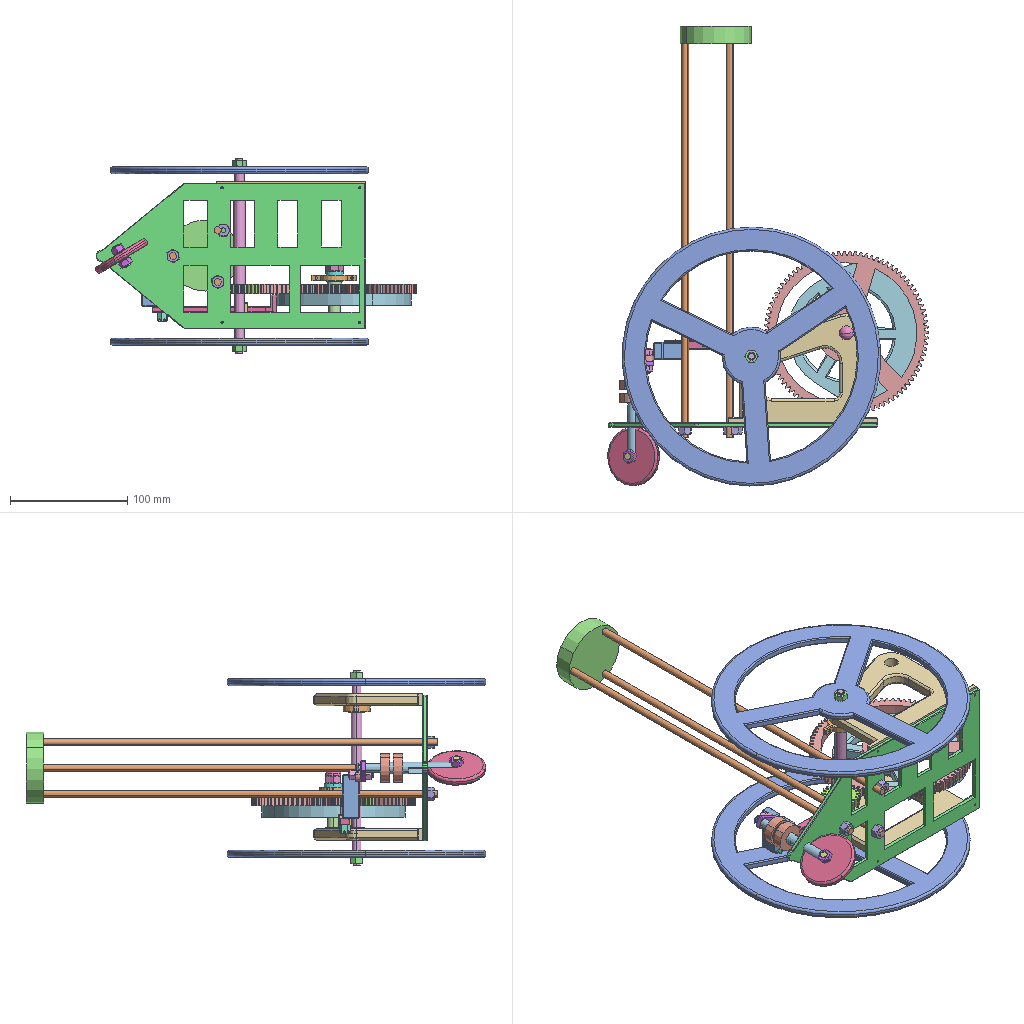Assembly | SolidWorks | 33 different items | 41 placed | box 273 x 391 x 166 mm
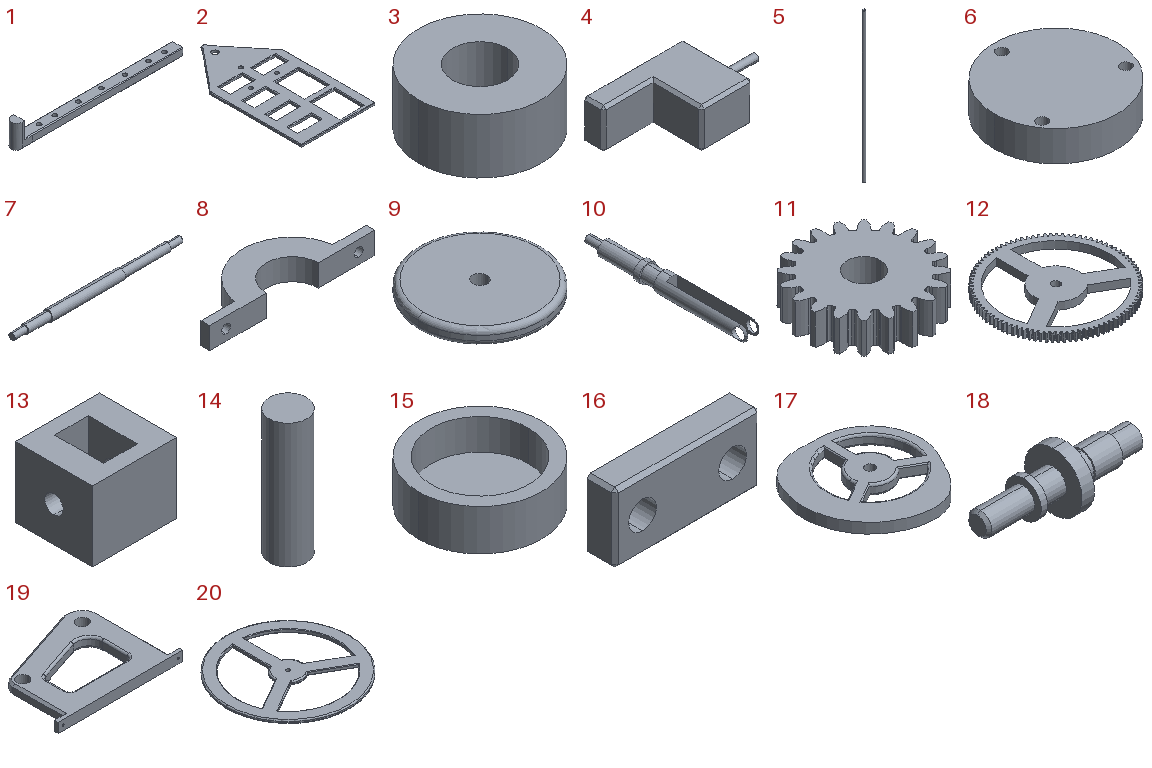Parts list (item | name | quantity | size | volume | features):
1 | - | x1 | 105.759 x 6.991 x 14.8 mm | 3589 mm3 | features Chamfer 1, Extrusion 1, Fillet 1, ICE 1
2 | - | x1 | 124.097 x 229.379 x 4 mm | 63027 mm3 | features Chamfer 8, Fillet 2, Extrusion 1, ICE 1
3 | - | x1 | 11.179 x 11.179 x 5 mm | 392.607 mm3 | features Extrusion 1
4 | - | x1 | 48 x 26.348 x 15 mm | 9753 mm3 | features Chamfer 1, Extrusion 1, ICE 1
5 | - | x3 | 6 x 6 x 350 mm | 9896 mm3 | features Extrusion 1
6 | - | x1 | 60.454 x 60.454 x 15 mm | 42106 mm3 | features Extrusion 1
7 | - | x1 | 166.354 x 10 x 10 mm | 9800 mm3 | features Revolution 1
8 | - | x4 | 38 x 11.5 x 5 mm | 894.544 mm3 | features ICE 2, Extrusion 1
9 | - | x1 | 50 x 50 x 6 mm | 11346 mm3 | features Extrusion 1, Fillet 1
10 | - | x1 | 10 x 90.414 x 10 mm | 3064 mm3 | features ICE 2, Revolution 1
11 | - | x1 | 32.74 x 32.74 x 8.27 mm | 5212 mm3 | features Extrusion 1
12 | - | x1 | 139.495 x 139.48 x 8.27 mm | 56874 mm3 | features Extrusion 1, ICE 1
13 | - | x1 | 11.98 x 10.98 x 10 mm | 942.243 mm3 | features Extrusion 1, ICE 1
14 | - | x1 | 6 x 6 x 20 mm | 565.487 mm3 | features Extrusion 1
15 | - | x2 | 24 x 24 x 8 mm | 1918 mm3 | features Extrusion 1, ICE 1
16 | - | x1 | 21 x 4 x 10 mm | 730.052 mm3 | features Chamfer 1, Extrusion 1, ICE 1
17 | - | x1 | 115.52 x 116.155 x 10 mm | 73313 mm3 | features Fillet 2, Chamfer 1, Extrusion 1, ICE 1
18 | - | x1 | 53.633 x 20 x 20 mm | 4453 mm3 | features Revolution 1
19 | - | x2 | 127.21 x 92.5 x 10 mm | 59705 mm3 | features Fillet 3, Chamfer 2, ICE 2, Extrusion 1
20 | - | x2 | 220.16 x 220.16 x 6 mm | 108989 mm3 | features Fillet 3, Chamfer 1, Extrusion 1, ICE 1
21 | angular contact ball bearings gb | x1 | - | - | -
22 | cross recessed ctsk head screws type b gb | x1 | - | - | -
23 | curved spring washers gb | x1 | - | - | -
24 | double end studs bm=1d gb | x1 | - | - | -
25 | hex nuts, style 1-grades ab gb | x1 | - | - | -
26 | hex nuts, style 2-grades ab gb | x1 | - | - | -
27 | hex slotted nuts style 1-grades c gb | x1 | - | - | -
28 | hex socket set screws with flat point gb | x1 | - | - | -
29 | lid nut gb | x1 | - | - | -
30 | miniature radial ball bearings gb | x1 | - | - | -
31 | prevailing torque hex nuts2 class 9 gb | x1 | - | - | -
32 | round nuts drilled holes in one face gb | x1 | - | - | -
33 | small hex thin nuts-fine pitch thread gb | x1 | - | - | -
Mates (type | each side: item.copy, entity, surface, feature):
Concentric | 20.1 edge | 7.1 edge
Concentric | 7.1 edge | 20.2 edge
Coincident | 7.1 face plane Revolve1 | 20.2 face plane Boss-Extrude2
Coincident | 20.1 face plane Boss-Extrude2 | 7.1 face plane Revolve1
Concentric | 11.1 edge | 7.1 edge
Coincident | 11.1 face plane Boss-Extrude1 | 7.1 face plane Revolve1
Parallel | 12.1 face plane Boss-Extrude1 | 20.1 face plane Boss-Extrude2
Concentric | 8.1 edge | 8.2 edge
Coincident | 8.1 face plane Boss-Extrude1 | 8.2 face plane Boss-Extrude1 | 2 times
Parallel | 8.2 face plane Boss-Extrude1 | assembly plane
Concentric | 9.1 edge | 10.1 edge
Coincident | 9.1 face plane Boss-Extrude1 | 10.1 face plane Cut-Extrude1
Concentric | 10.1 edge | 14.1 edge
DistanceDim | 14.1 face plane Boss-Extrude1 | 9.1 face plane Boss-Extrude1
Coincident | 10.1 face plane Revolve1 | 15.1 face plane Boss-Extrude1
Concentric | 12.1 edge | 18.1 edge
Coincident | 12.1 face plane Boss-Extrude1 | 18.1 face plane Revolve1
Coincident | 8.3 face plane Boss-Extrude1 | 8.4 face plane Boss-Extrude1 | 2 times
Concentric | 8.3 edge | 8.4 edge
Coincident | assembly face | assembly face | 8 times
Concentric | assembly edge | assembly edge | 8 times
Coincident | assembly edge | assembly face | 3 times
Concentric | 18.1 edge | 19.1 edge
Concentric | 7.1 edge | 19.1 edge
Coincident | 18.1 edge | 19.1 face plane Boss-Extrude1
Parallel | 19.1 face plane Boss-Extrude1 | assembly plane
Concentric | 10.1 edge | 16.1 edge
Tangent | 20.1 face cylinder Boss-Extrude2 | assembly plane
Tangent | 9.1 face cylinder Boss-Extrude1 | assembly plane
Parallel | 15.2 face plane Boss-Extrude1 | 2.1 face plane Boss-Extrude1
Coincident | 19.1 face plane Boss-Extrude1 | 2.1 face plane Boss-Extrude1 | 2 times
Parallel | 20.2 face plane Boss-Extrude2 | 2.1 face plane Boss-Extrude1
Concentric | 15.1 edge | 2.1 edge
Parallel | 2.1 face plane Boss-Extrude1 | 4.1 face plane Boss-Extrude1
Concentric | 2.1 edge | 5.1 edge
Concentric | 2.1 edge | 5.2 edge
Concentric | 2.1 edge | 5.3 edge
Concentric | 5.2 edge | 6.1 edge
Coincident | 5.3 face plane Boss-Extrude1 | 6.1 face plane Boss-Extrude1
Concentric | 5.1 edge | 6.1 edge
Coincident | 4.1 face plane Boss-Extrude1 | 1.1 face plane
Concentric | 4.1 edge | 1.1 edge
Concentric | 18.1 edge | 17.1 edge
Coincident | 18.1 face plane Revolve1 | 17.1 face plane Boss-Extrude1
CamTangent | 17.1 face surface:4009 Boss-Extrude1 | 1.1 face cylinder
Parallel | 1.1 face plane | 17.1 face plane Boss-Extrude1
DistanceDim | 1.1 face plane | 17.1 face plane Boss-Extrude1
DistanceDim | 4.1 face plane Boss-Extrude1 | 3.1 face plane Boss-Extrude1
Parallel | 1.1 face plane | 13.1 face plane | 2 times
Coincident | 13.1 face plane | 19.1 face plane Boss-Extrude1
Concentric | 10.1 face cylinder Revolve1 | 16.1 edge
Coincident | 10.1 face plane Revolve1 | 16.1 face plane Boss-Extrude1
Coincident | 1.1 face plane | 13.1 face plane
Parallel | 2.1 face plane Boss-Extrude1 | 1.1 face plane
DistanceDim | 1.1 face plane | 2.1 face plane Boss-Extrude1
Concentric | 3.1 face cylinder Boss-Extrude1 | 16.1 edge
DistanceDim | 13.1 face plane | 19.1 face plane Boss-Extrude1
GearDim | 12.1 edge | 11.1 edge
Coincident | 12.1 face plane Boss-Extrude1 | 11.1 face plane Boss-Extrude1
Concentric | 10.1 edge | 15.2 edge
DistanceDim | 20.2 face plane Boss-Extrude2 | 2.1 face plane Boss-Extrude1
Tangent | 3.1 face cylinder Boss-Extrude1 | 4.1 face plane Boss-Extrude1